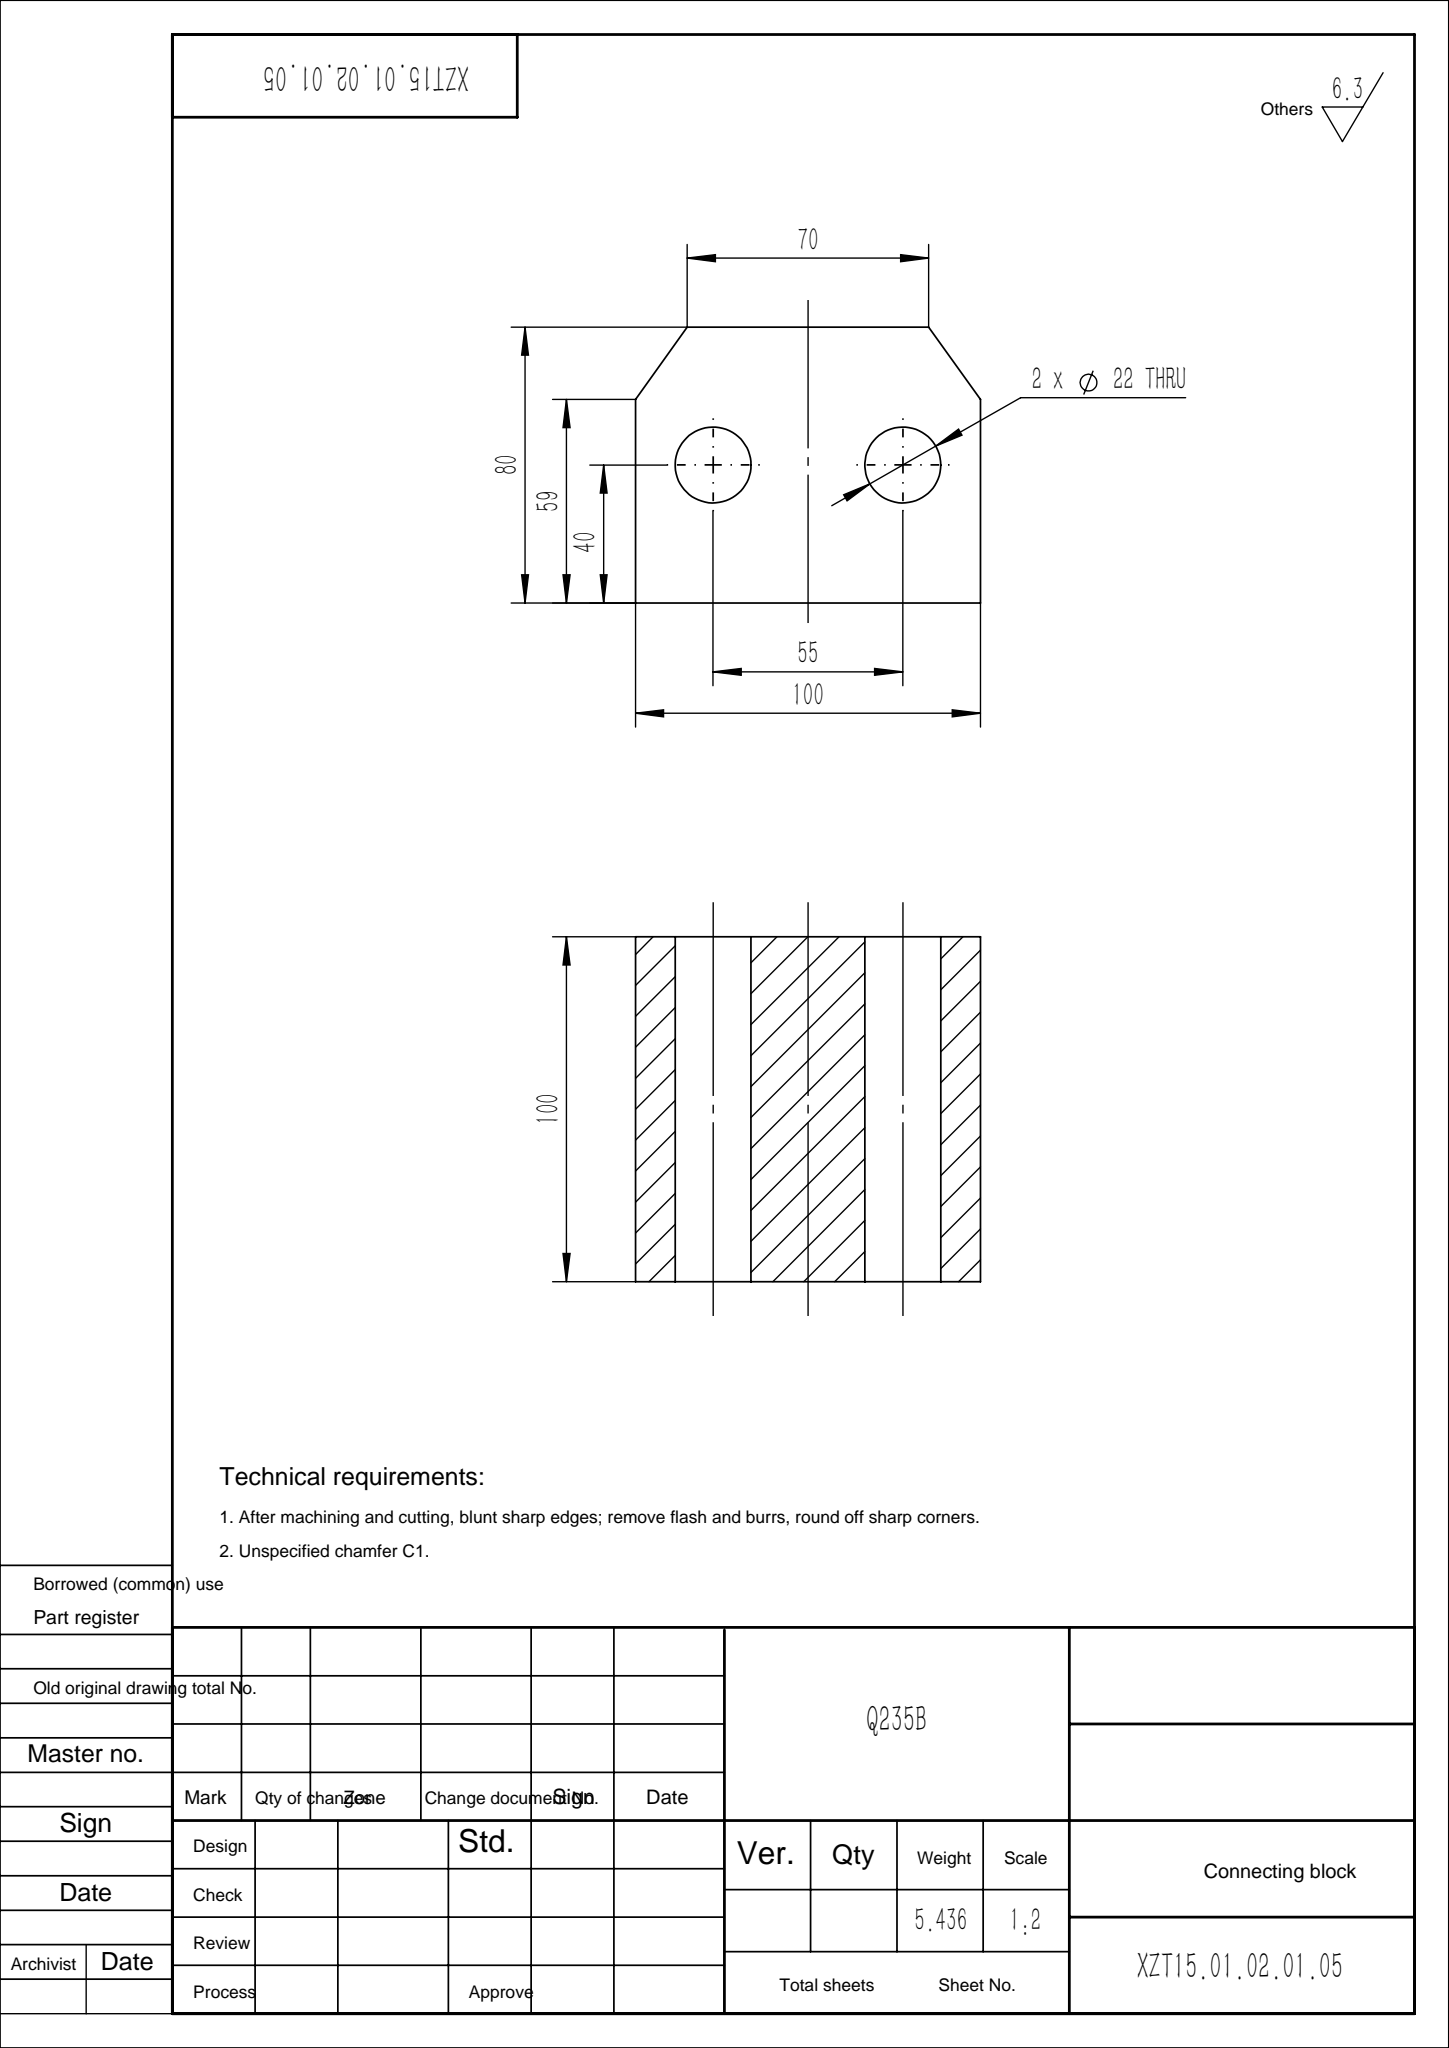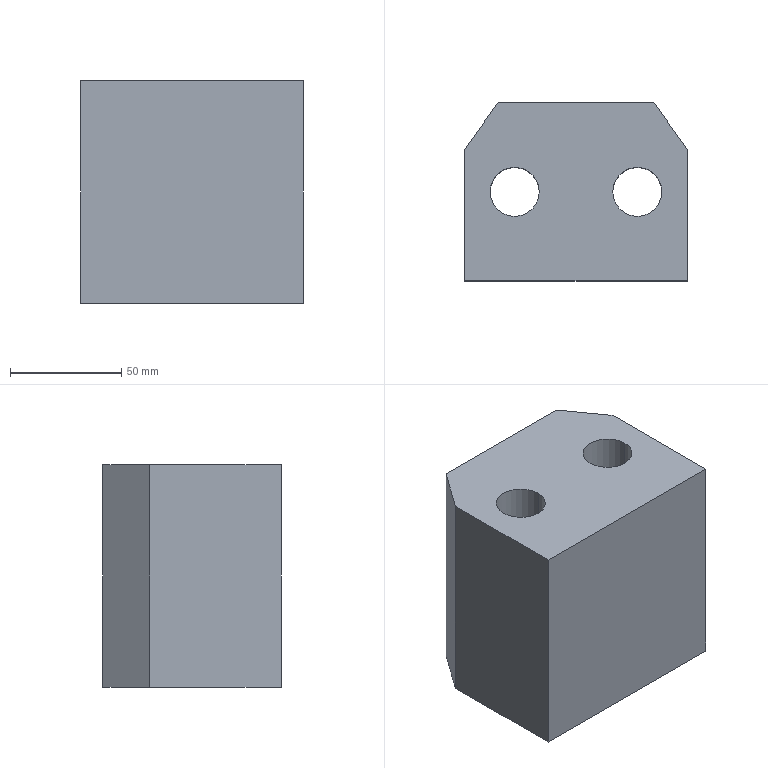Part | SolidWorks | features Chamfer 1, Extrusion 1, HoleWzd 1, ICE 1 | 1 solid | 12 faces | box 100 x 80 x 100 mm | volume 692473 mm3 | plane 8 | cylinder 4 | commonest cylinder face diameters 22 x4
STEP:
#1=CARTESIAN_POINT('',(-38.5,0.,0.));
#2=VERTEX_POINT('',#1);
#3=CARTESIAN_POINT('',(-16.5,0.,0.));
#4=VERTEX_POINT('',#3);
#5=CARTESIAN_POINT('',(-27.5,0.,0.));
#6=DIRECTION('',(0.,0.,1.));
#7=DIRECTION('',(1.,0.,0.));
#8=AXIS2_PLACEMENT_3D('',#5,#6,#7);
#9=CIRCLE('',#8,11.);
#10=EDGE_CURVE('',#2,#4,#9,.T.);
#11=ORIENTED_EDGE('',*,*,#10,.F.);
#12=CARTESIAN_POINT('',(-38.5,0.,100.));
#13=VERTEX_POINT('',#12);
#14=CARTESIAN_POINT('',(-38.5,0.,100.));
#15=DIRECTION('',(0.,0.,1.));
#16=VECTOR('',#15,1000.);
#17=LINE('',#14,#16);
#18=EDGE_CURVE('',#2,#13,#17,.T.);
#19=ORIENTED_EDGE('',*,*,#18,.T.);
#20=CARTESIAN_POINT('',(-16.5,0.,100.));
#21=VERTEX_POINT('',#20);
#22=CARTESIAN_POINT('',(-27.5,0.,100.));
#23=DIRECTION('',(0.,0.,1.));
#24=DIRECTION('',(1.,0.,0.));
#25=AXIS2_PLACEMENT_3D('',#22,#23,#24);
#26=CIRCLE('',#25,11.);
#27=EDGE_CURVE('',#13,#21,#26,.T.);
#28=ORIENTED_EDGE('',*,*,#27,.T.);
#29=CARTESIAN_POINT('',(-16.5,0.,100.));
#30=DIRECTION('',(0.,0.,1.));
#31=VECTOR('',#30,1000.);
#32=LINE('',#29,#31);
#33=EDGE_CURVE('',#4,#21,#32,.T.);
#34=ORIENTED_EDGE('',*,*,#33,.F.);
#35=EDGE_LOOP('',(#11,#19,#28,#34));
#36=FACE_OUTER_BOUND('',#35,.T.);
#37=CARTESIAN_POINT('',(-27.5,0.,100.));
#38=DIRECTION('',(0.,0.,1.));
#39=DIRECTION('',(1.,0.,0.));
#40=AXIS2_PLACEMENT_3D('',#37,#38,#39);
#41=CYLINDRICAL_SURFACE('',#40,11.);
#42=ADVANCED_FACE('',(#36),#41,.F.);
#43=CARTESIAN_POINT('',(16.5,0.,0.));
#44=VERTEX_POINT('',#43);
#45=CARTESIAN_POINT('',(38.5,0.,0.));
#46=VERTEX_POINT('',#45);
#47=CARTESIAN_POINT('',(27.5,0.,0.));
#48=DIRECTION('',(0.,0.,1.));
#49=DIRECTION('',(1.,0.,0.));
#50=AXIS2_PLACEMENT_3D('',#47,#48,#49);
#51=CIRCLE('',#50,11.);
#52=EDGE_CURVE('',#44,#46,#51,.T.);
#53=ORIENTED_EDGE('',*,*,#52,.F.);
#54=CARTESIAN_POINT('',(16.5,0.,100.));
#55=VERTEX_POINT('',#54);
#56=CARTESIAN_POINT('',(16.5,0.,100.));
#57=DIRECTION('',(0.,0.,1.));
#58=VECTOR('',#57,1000.);
#59=LINE('',#56,#58);
#60=EDGE_CURVE('',#44,#55,#59,.T.);
#61=ORIENTED_EDGE('',*,*,#60,.T.);
#62=CARTESIAN_POINT('',(38.5,0.,100.));
#63=VERTEX_POINT('',#62);
#64=CARTESIAN_POINT('',(27.5,0.,100.));
#65=DIRECTION('',(0.,0.,1.));
#66=DIRECTION('',(1.,0.,0.));
#67=AXIS2_PLACEMENT_3D('',#64,#65,#66);
#68=CIRCLE('',#67,11.);
#69=EDGE_CURVE('',#55,#63,#68,.T.);
#70=ORIENTED_EDGE('',*,*,#69,.T.);
#71=CARTESIAN_POINT('',(38.5,0.,100.));
#72=DIRECTION('',(0.,0.,1.));
#73=VECTOR('',#72,1000.);
#74=LINE('',#71,#73);
#75=EDGE_CURVE('',#46,#63,#74,.T.);
#76=ORIENTED_EDGE('',*,*,#75,.F.);
#77=EDGE_LOOP('',(#53,#61,#70,#76));
#78=FACE_OUTER_BOUND('',#77,.T.);
#79=CARTESIAN_POINT('',(27.5,0.,100.));
#80=DIRECTION('',(0.,0.,1.));
#81=DIRECTION('',(1.,0.,0.));
#82=AXIS2_PLACEMENT_3D('',#79,#80,#81);
#83=CYLINDRICAL_SURFACE('',#82,11.);
#84=ADVANCED_FACE('',(#78),#83,.F.);
#85=CARTESIAN_POINT('',(-50.,19.,100.));
#86=VERTEX_POINT('',#85);
#87=CARTESIAN_POINT('',(-50.,-40.,100.));
#88=VERTEX_POINT('',#87);
#89=CARTESIAN_POINT('',(-50.,-40.,100.));
#90=DIRECTION('',(0.,-1.,0.));
#91=VECTOR('',#90,1000.);
#92=LINE('',#89,#91);
#93=EDGE_CURVE('',#86,#88,#92,.T.);
#94=ORIENTED_EDGE('',*,*,#93,.F.);
#95=CARTESIAN_POINT('',(-50.,19.,0.));
#96=VERTEX_POINT('',#95);
#97=CARTESIAN_POINT('',(-50.,19.,0.));
#98=DIRECTION('',(0.,0.,1.));
#99=VECTOR('',#98,1000.);
#100=LINE('',#97,#99);
#101=EDGE_CURVE('',#96,#86,#100,.T.);
#102=ORIENTED_EDGE('',*,*,#101,.F.);
#103=CARTESIAN_POINT('',(-50.,-40.,0.));
#104=VERTEX_POINT('',#103);
#105=CARTESIAN_POINT('',(-50.,-40.,0.));
#106=DIRECTION('',(0.,-1.,0.));
#107=VECTOR('',#106,1000.);
#108=LINE('',#105,#107);
#109=EDGE_CURVE('',#96,#104,#108,.T.);
#110=ORIENTED_EDGE('',*,*,#109,.T.);
#111=CARTESIAN_POINT('',(-50.,-40.,100.));
#112=DIRECTION('',(0.,0.,-1.));
#113=VECTOR('',#112,1000.);
#114=LINE('',#111,#113);
#115=EDGE_CURVE('',#88,#104,#114,.T.);
#116=ORIENTED_EDGE('',*,*,#115,.F.);
#117=EDGE_LOOP('',(#94,#102,#110,#116));
#118=FACE_OUTER_BOUND('',#117,.T.);
#119=CARTESIAN_POINT('',(-50.,-40.,100.));
#120=DIRECTION('',(1.,0.,0.));
#121=DIRECTION('',(0.,0.,-1.));
#122=AXIS2_PLACEMENT_3D('',#119,#120,#121);
#123=PLANE('',#122);
#124=ADVANCED_FACE('',(#118),#123,.F.);
#125=CARTESIAN_POINT('',(50.,-40.,0.));
#126=VERTEX_POINT('',#125);
#127=CARTESIAN_POINT('',(50.,-40.,0.));
#128=DIRECTION('',(1.,0.,0.));
#129=VECTOR('',#128,1000.);
#130=LINE('',#127,#129);
#131=EDGE_CURVE('',#104,#126,#130,.T.);
#132=ORIENTED_EDGE('',*,*,#131,.T.);
#133=CARTESIAN_POINT('',(50.,-40.,100.));
#134=VERTEX_POINT('',#133);
#135=CARTESIAN_POINT('',(50.,-40.,100.));
#136=DIRECTION('',(0.,0.,-1.));
#137=VECTOR('',#136,1000.);
#138=LINE('',#135,#137);
#139=EDGE_CURVE('',#134,#126,#138,.T.);
#140=ORIENTED_EDGE('',*,*,#139,.F.);
#141=CARTESIAN_POINT('',(50.,-40.,100.));
#142=DIRECTION('',(1.,0.,0.));
#143=VECTOR('',#142,1000.);
#144=LINE('',#141,#143);
#145=EDGE_CURVE('',#88,#134,#144,.T.);
#146=ORIENTED_EDGE('',*,*,#145,.F.);
#147=ORIENTED_EDGE('',*,*,#115,.T.);
#148=EDGE_LOOP('',(#132,#140,#146,#147));
#149=FACE_OUTER_BOUND('',#148,.T.);
#150=CARTESIAN_POINT('',(50.,-40.,100.));
#151=DIRECTION('',(0.,1.,0.));
#152=DIRECTION('',(-1.,0.,0.));
#153=AXIS2_PLACEMENT_3D('',#150,#151,#152);
#154=PLANE('',#153);
#155=ADVANCED_FACE('',(#149),#154,.F.);
#156=CARTESIAN_POINT('',(50.,19.,0.));
#157=VERTEX_POINT('',#156);
#158=CARTESIAN_POINT('',(50.,-40.,0.));
#159=DIRECTION('',(0.,1.,0.));
#160=VECTOR('',#159,1000.);
#161=LINE('',#158,#160);
#162=EDGE_CURVE('',#126,#157,#161,.T.);
#163=ORIENTED_EDGE('',*,*,#162,.T.);
#164=CARTESIAN_POINT('',(50.,19.,100.));
#165=VERTEX_POINT('',#164);
#166=CARTESIAN_POINT('',(50.,19.,0.));
#167=DIRECTION('',(0.,0.,1.));
#168=VECTOR('',#167,1000.);
#169=LINE('',#166,#168);
#170=EDGE_CURVE('',#157,#165,#169,.T.);
#171=ORIENTED_EDGE('',*,*,#170,.T.);
#172=CARTESIAN_POINT('',(50.,-40.,100.));
#173=DIRECTION('',(0.,1.,0.));
#174=VECTOR('',#173,1000.);
#175=LINE('',#172,#174);
#176=EDGE_CURVE('',#134,#165,#175,.T.);
#177=ORIENTED_EDGE('',*,*,#176,.F.);
#178=ORIENTED_EDGE('',*,*,#139,.T.);
#179=EDGE_LOOP('',(#163,#171,#177,#178));
#180=FACE_OUTER_BOUND('',#179,.T.);
#181=CARTESIAN_POINT('',(50.,-40.,100.));
#182=DIRECTION('',(-1.,0.,0.));
#183=DIRECTION('',(0.,0.,1.));
#184=AXIS2_PLACEMENT_3D('',#181,#182,#183);
#185=PLANE('',#184);
#186=ADVANCED_FACE('',(#180),#185,.F.);
#187=CARTESIAN_POINT('',(35.,40.,0.));
#188=VERTEX_POINT('',#187);
#189=CARTESIAN_POINT('',(-35.,40.,0.));
#190=VERTEX_POINT('',#189);
#191=CARTESIAN_POINT('',(50.,40.,0.));
#192=DIRECTION('',(-1.,0.,0.));
#193=VECTOR('',#192,1000.);
#194=LINE('',#191,#193);
#195=EDGE_CURVE('',#188,#190,#194,.T.);
#196=ORIENTED_EDGE('',*,*,#195,.T.);
#197=CARTESIAN_POINT('',(-35.,40.,100.));
#198=VERTEX_POINT('',#197);
#199=CARTESIAN_POINT('',(-35.,40.,0.));
#200=DIRECTION('',(0.,0.,1.));
#201=VECTOR('',#200,1000.);
#202=LINE('',#199,#201);
#203=EDGE_CURVE('',#190,#198,#202,.T.);
#204=ORIENTED_EDGE('',*,*,#203,.T.);
#205=CARTESIAN_POINT('',(35.,40.,100.));
#206=VERTEX_POINT('',#205);
#207=CARTESIAN_POINT('',(50.,40.,100.));
#208=DIRECTION('',(-1.,0.,0.));
#209=VECTOR('',#208,1000.);
#210=LINE('',#207,#209);
#211=EDGE_CURVE('',#206,#198,#210,.T.);
#212=ORIENTED_EDGE('',*,*,#211,.F.);
#213=CARTESIAN_POINT('',(35.,40.,0.));
#214=DIRECTION('',(0.,0.,1.));
#215=VECTOR('',#214,1000.);
#216=LINE('',#213,#215);
#217=EDGE_CURVE('',#188,#206,#216,.T.);
#218=ORIENTED_EDGE('',*,*,#217,.F.);
#219=EDGE_LOOP('',(#196,#204,#212,#218));
#220=FACE_OUTER_BOUND('',#219,.T.);
#221=CARTESIAN_POINT('',(50.,40.,100.));
#222=DIRECTION('',(0.,-1.,0.));
#223=DIRECTION('',(1.,0.,0.));
#224=AXIS2_PLACEMENT_3D('',#221,#222,#223);
#225=PLANE('',#224);
#226=ADVANCED_FACE('',(#220),#225,.F.);
#227=CARTESIAN_POINT('',(-42.095,30.068,100.));
#228=DIRECTION('',(0.5812,0.8137,0.));
#229=VECTOR('',#228,1000.);
#230=LINE('',#227,#229);
#231=EDGE_CURVE('',#86,#198,#230,.T.);
#232=ORIENTED_EDGE('',*,*,#231,.F.);
#233=ORIENTED_EDGE('',*,*,#93,.T.);
#234=ORIENTED_EDGE('',*,*,#145,.T.);
#235=ORIENTED_EDGE('',*,*,#176,.T.);
#236=CARTESIAN_POINT('',(42.095,30.068,100.));
#237=DIRECTION('',(0.5812,-0.8137,0.));
#238=VECTOR('',#237,1000.);
#239=LINE('',#236,#238);
#240=EDGE_CURVE('',#206,#165,#239,.T.);
#241=ORIENTED_EDGE('',*,*,#240,.F.);
#242=ORIENTED_EDGE('',*,*,#211,.T.);
#243=EDGE_LOOP('',(#232,#233,#234,#235,#241,#242));
#244=FACE_OUTER_BOUND('',#243,.T.);
#245=CARTESIAN_POINT('',(-27.5,0.,100.));
#246=DIRECTION('',(0.,0.,1.));
#247=DIRECTION('',(1.,0.,0.));
#248=AXIS2_PLACEMENT_3D('',#245,#246,#247);
#249=CIRCLE('',#248,11.);
#250=EDGE_CURVE('',#21,#13,#249,.T.);
#251=ORIENTED_EDGE('',*,*,#250,.F.);
#252=ORIENTED_EDGE('',*,*,#27,.F.);
#253=EDGE_LOOP('',(#251,#252));
#254=FACE_BOUND('',#253,.T.);
#255=CARTESIAN_POINT('',(27.5,0.,100.));
#256=DIRECTION('',(0.,0.,1.));
#257=DIRECTION('',(1.,0.,0.));
#258=AXIS2_PLACEMENT_3D('',#255,#256,#257);
#259=CIRCLE('',#258,11.);
#260=EDGE_CURVE('',#63,#55,#259,.T.);
#261=ORIENTED_EDGE('',*,*,#260,.F.);
#262=ORIENTED_EDGE('',*,*,#69,.F.);
#263=EDGE_LOOP('',(#261,#262));
#264=FACE_BOUND('',#263,.T.);
#265=CARTESIAN_POINT('',(0.,0.,100.));
#266=DIRECTION('',(0.,0.,1.));
#267=DIRECTION('',(1.,0.,0.));
#268=AXIS2_PLACEMENT_3D('',#265,#266,#267);
#269=PLANE('',#268);
#270=ADVANCED_FACE('',(#244,#254,#264),#269,.T.);
#271=CARTESIAN_POINT('',(-27.5,0.,0.));
#272=DIRECTION('',(0.,0.,1.));
#273=DIRECTION('',(1.,0.,0.));
#274=AXIS2_PLACEMENT_3D('',#271,#272,#273);
#275=CIRCLE('',#274,11.);
#276=EDGE_CURVE('',#4,#2,#275,.T.);
#277=ORIENTED_EDGE('',*,*,#276,.T.);
#278=ORIENTED_EDGE('',*,*,#10,.T.);
#279=EDGE_LOOP('',(#277,#278));
#280=FACE_BOUND('',#279,.T.);
#281=CARTESIAN_POINT('',(27.5,0.,0.));
#282=DIRECTION('',(0.,0.,1.));
#283=DIRECTION('',(1.,0.,0.));
#284=AXIS2_PLACEMENT_3D('',#281,#282,#283);
#285=CIRCLE('',#284,11.);
#286=EDGE_CURVE('',#46,#44,#285,.T.);
#287=ORIENTED_EDGE('',*,*,#286,.T.);
#288=ORIENTED_EDGE('',*,*,#52,.T.);
#289=EDGE_LOOP('',(#287,#288));
#290=FACE_BOUND('',#289,.T.);
#291=ORIENTED_EDGE('',*,*,#109,.F.);
#292=CARTESIAN_POINT('',(-35.,40.,0.));
#293=DIRECTION('',(0.5812,0.8137,0.));
#294=VECTOR('',#293,1000.);
#295=LINE('',#292,#294);
#296=EDGE_CURVE('',#96,#190,#295,.T.);
#297=ORIENTED_EDGE('',*,*,#296,.T.);
#298=ORIENTED_EDGE('',*,*,#195,.F.);
#299=CARTESIAN_POINT('',(35.,40.,0.));
#300=DIRECTION('',(0.5812,-0.8137,0.));
#301=VECTOR('',#300,1000.);
#302=LINE('',#299,#301);
#303=EDGE_CURVE('',#188,#157,#302,.T.);
#304=ORIENTED_EDGE('',*,*,#303,.T.);
#305=ORIENTED_EDGE('',*,*,#162,.F.);
#306=ORIENTED_EDGE('',*,*,#131,.F.);
#307=EDGE_LOOP('',(#291,#297,#298,#304,#305,#306));
#308=FACE_OUTER_BOUND('',#307,.T.);
#309=CARTESIAN_POINT('',(0.,0.,0.));
#310=DIRECTION('',(0.,0.,1.));
#311=DIRECTION('',(1.,0.,0.));
#312=AXIS2_PLACEMENT_3D('',#309,#310,#311);
#313=PLANE('',#312);
#314=ADVANCED_FACE('',(#280,#290,#308),#313,.F.);
#315=ORIENTED_EDGE('',*,*,#60,.F.);
#316=ORIENTED_EDGE('',*,*,#286,.F.);
#317=ORIENTED_EDGE('',*,*,#75,.T.);
#318=ORIENTED_EDGE('',*,*,#260,.T.);
#319=EDGE_LOOP('',(#315,#316,#317,#318));
#320=FACE_OUTER_BOUND('',#319,.T.);
#321=CARTESIAN_POINT('',(27.5,0.,100.));
#322=DIRECTION('',(0.,0.,1.));
#323=DIRECTION('',(1.,0.,0.));
#324=AXIS2_PLACEMENT_3D('',#321,#322,#323);
#325=CYLINDRICAL_SURFACE('',#324,11.);
#326=ADVANCED_FACE('',(#320),#325,.F.);
#327=ORIENTED_EDGE('',*,*,#18,.F.);
#328=ORIENTED_EDGE('',*,*,#276,.F.);
#329=ORIENTED_EDGE('',*,*,#33,.T.);
#330=ORIENTED_EDGE('',*,*,#250,.T.);
#331=EDGE_LOOP('',(#327,#328,#329,#330));
#332=FACE_OUTER_BOUND('',#331,.T.);
#333=CARTESIAN_POINT('',(-27.5,0.,100.));
#334=DIRECTION('',(0.,0.,1.));
#335=DIRECTION('',(1.,0.,0.));
#336=AXIS2_PLACEMENT_3D('',#333,#334,#335);
#337=CYLINDRICAL_SURFACE('',#336,11.);
#338=ADVANCED_FACE('',(#332),#337,.F.);
#339=ORIENTED_EDGE('',*,*,#240,.T.);
#340=ORIENTED_EDGE('',*,*,#170,.F.);
#341=ORIENTED_EDGE('',*,*,#303,.F.);
#342=ORIENTED_EDGE('',*,*,#217,.T.);
#343=EDGE_LOOP('',(#339,#340,#341,#342));
#344=FACE_OUTER_BOUND('',#343,.T.);
#345=CARTESIAN_POINT('',(35.,40.,0.));
#346=DIRECTION('',(-0.8137,-0.5812,0.));
#347=DIRECTION('',(0.5812,-0.8137,0.));
#348=AXIS2_PLACEMENT_3D('',#345,#346,#347);
#349=PLANE('',#348);
#350=ADVANCED_FACE('',(#344),#349,.F.);
#351=ORIENTED_EDGE('',*,*,#231,.T.);
#352=ORIENTED_EDGE('',*,*,#203,.F.);
#353=ORIENTED_EDGE('',*,*,#296,.F.);
#354=ORIENTED_EDGE('',*,*,#101,.T.);
#355=EDGE_LOOP('',(#351,#352,#353,#354));
#356=FACE_OUTER_BOUND('',#355,.T.);
#357=CARTESIAN_POINT('',(-35.,40.,0.));
#358=DIRECTION('',(0.8137,-0.5812,0.));
#359=DIRECTION('',(0.5812,0.8137,0.));
#360=AXIS2_PLACEMENT_3D('',#357,#358,#359);
#361=PLANE('',#360);
#362=ADVANCED_FACE('',(#356),#361,.F.);
#363=CLOSED_SHELL('',(#42,#84,#124,#155,#186,#226,#270,#314,#326,#338,#350,#362));
#364=MANIFOLD_SOLID_BREP('',#363);
#365=CARTESIAN_POINT('',(0.,0.,0.));
#366=DIRECTION('',(0.,0.,1.));
#367=DIRECTION('',(1.,0.,0.));
#368=AXIS2_PLACEMENT_3D('',#365,#366,#367);
#369=(LENGTH_UNIT()NAMED_UNIT(*)SI_UNIT(.MILLI.,.METRE.));
#370=UNCERTAINTY_MEASURE_WITH_UNIT(LENGTH_MEASURE(0.00001),#369,'','');
#371=(NAMED_UNIT(*)PLANE_ANGLE_UNIT()SI_UNIT($,.RADIAN.));
#372=(NAMED_UNIT(*)SI_UNIT($,.STERADIAN.)SOLID_ANGLE_UNIT());
#373=(GEOMETRIC_REPRESENTATION_CONTEXT(3)GLOBAL_UNCERTAINTY_ASSIGNED_CONTEXT((#370))GLOBAL_UNIT_ASSIGNED_CONTEXT((#369,#371,#372))REPRESENTATION_CONTEXT('',''));
#374=ADVANCED_BREP_SHAPE_REPRESENTATION('',(#364,#368),#373);